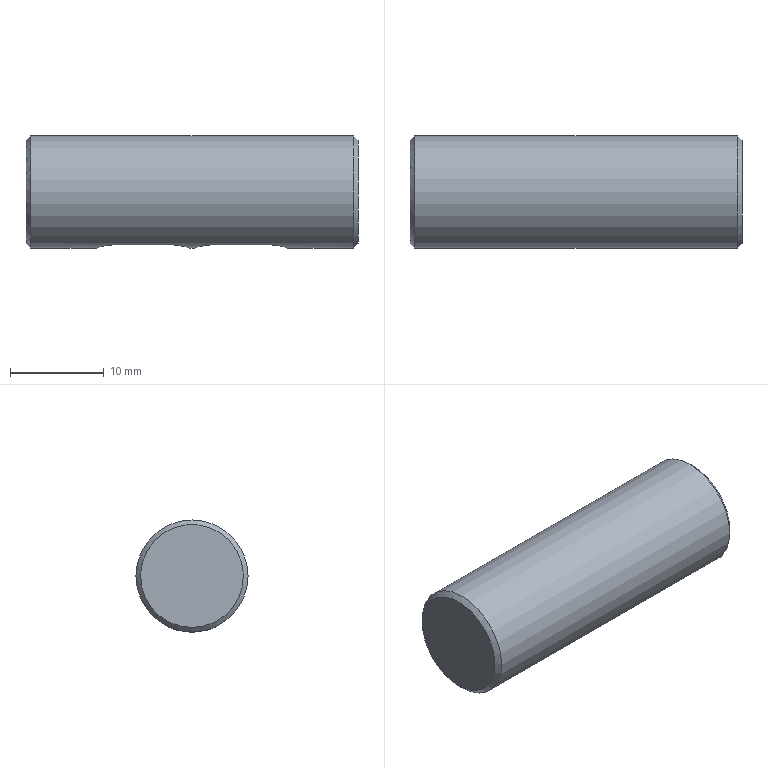Part | NX | features BREP 1 | 1 solid | 15 faces | box 35.5 x 12 x 12 mm | volume 3831 mm3 | plane 8 | cylinder 5 | cone 2 | commonest cylinder face diameters 4 x4 12 x1
STEP:
#1=CARTESIAN_POINT('',(0.5,0.,-6.));
#2=VERTEX_POINT('',#1);
#3=CARTESIAN_POINT('',(0.5,0.,0.));
#4=DIRECTION('',(1.,0.,0.));
#5=DIRECTION('',(0.,0.,-1.));
#6=AXIS2_PLACEMENT_3D('',#3,#4,#5);
#7=CIRCLE('',#6,6.);
#8=EDGE_CURVE('',#2,#2,#7,.T.);
#9=ORIENTED_EDGE('',*,*,#8,.F.);
#10=EDGE_LOOP('',(#9));
#11=FACE_BOUND('',#10,.T.);
#12=CARTESIAN_POINT('',(0.,0.,-5.5));
#13=VERTEX_POINT('',#12);
#14=CARTESIAN_POINT('',(0.,0.,0.));
#15=DIRECTION('',(-1.,0.,0.));
#16=DIRECTION('',(0.,0.,-1.));
#17=AXIS2_PLACEMENT_3D('',#14,#15,#16);
#18=CIRCLE('',#17,5.5);
#19=EDGE_CURVE('',#13,#13,#18,.T.);
#20=ORIENTED_EDGE('',*,*,#19,.F.);
#21=EDGE_LOOP('',(#20));
#22=FACE_BOUND('',#21,.T.);
#23=CARTESIAN_POINT('',(0.,0.,0.));
#24=DIRECTION('',(1.,0.,0.));
#25=DIRECTION('',(0.,0.,-1.));
#26=AXIS2_PLACEMENT_3D('',#23,#24,#25);
#27=CONICAL_SURFACE('',#26,5.5,0.7854);
#28=ADVANCED_FACE('',(#11,#22),#27,.T.);
#29=CARTESIAN_POINT('',(35.,0.,6.));
#30=VERTEX_POINT('',#29);
#31=CARTESIAN_POINT('',(35.,0.,0.));
#32=DIRECTION('',(-1.,0.,0.));
#33=DIRECTION('',(0.,0.,1.));
#34=AXIS2_PLACEMENT_3D('',#31,#32,#33);
#35=CIRCLE('',#34,6.);
#36=EDGE_CURVE('',#30,#30,#35,.T.);
#37=ORIENTED_EDGE('',*,*,#36,.F.);
#38=EDGE_LOOP('',(#37));
#39=FACE_BOUND('',#38,.T.);
#40=CARTESIAN_POINT('',(35.5,0.,5.5));
#41=VERTEX_POINT('',#40);
#42=CARTESIAN_POINT('',(35.5,0.,0.));
#43=DIRECTION('',(1.,0.,0.));
#44=DIRECTION('',(0.,0.,1.));
#45=AXIS2_PLACEMENT_3D('',#42,#43,#44);
#46=CIRCLE('',#45,5.5);
#47=EDGE_CURVE('',#41,#41,#46,.T.);
#48=ORIENTED_EDGE('',*,*,#47,.F.);
#49=EDGE_LOOP('',(#48));
#50=FACE_BOUND('',#49,.T.);
#51=CARTESIAN_POINT('',(35.,0.,0.));
#52=DIRECTION('',(-1.,0.,0.));
#53=DIRECTION('',(0.,0.,1.));
#54=AXIS2_PLACEMENT_3D('',#51,#52,#53);
#55=CONICAL_SURFACE('',#54,6.,0.7854);
#56=ADVANCED_FACE('',(#39,#50),#55,.T.);
#57=CARTESIAN_POINT('',(20.,-2.,-3.5));
#58=VERTEX_POINT('',#57);
#59=CARTESIAN_POINT('',(20.,2.,-3.5));
#60=VERTEX_POINT('',#59);
#61=CARTESIAN_POINT('',(20.,0.,-3.5));
#62=DIRECTION('',(0.,0.,-1.));
#63=DIRECTION('',(1.,0.,0.));
#64=AXIS2_PLACEMENT_3D('',#61,#62,#63);
#65=CIRCLE('',#64,2.);
#66=EDGE_CURVE('',#58,#60,#65,.T.);
#67=ORIENTED_EDGE('',*,*,#66,.F.);
#68=CARTESIAN_POINT('',(20.,-2.,-5.657));
#69=VERTEX_POINT('',#68);
#70=CARTESIAN_POINT('',(20.,-2.,-3.5));
#71=DIRECTION('',(0.,0.,-1.));
#72=VECTOR('',#71,1000.);
#73=LINE('',#70,#72);
#74=EDGE_CURVE('',#58,#69,#73,.T.);
#75=ORIENTED_EDGE('',*,*,#74,.T.);
#76=CARTESIAN_POINT('',(20.,2.,-5.657));
#77=VERTEX_POINT('',#76);
#78=CARTESIAN_POINT('',(20.,2.,-5.657));
#79=CARTESIAN_POINT('',(19.467,2.,-5.657));
#80=CARTESIAN_POINT('',(18.438,1.567,-5.833));
#81=CARTESIAN_POINT('',(17.781,0.003461,-6.083));
#82=CARTESIAN_POINT('',(18.437,-1.568,-5.834));
#83=CARTESIAN_POINT('',(19.467,-2.,-5.657));
#84=CARTESIAN_POINT('',(20.,-2.,-5.657));
#85=B_SPLINE_CURVE_WITH_KNOTS('',3,(#78,#79,#80,#81,#82,#83,#84),.UNSPECIFIED.,.F.,.F.,(4,1,1,1,4),(0.,0.001574,0.003148,0.004722,0.006296),.UNSPECIFIED.);
#86=EDGE_CURVE('',#77,#69,#85,.T.);
#87=ORIENTED_EDGE('',*,*,#86,.F.);
#88=CARTESIAN_POINT('',(20.,2.,-3.5));
#89=DIRECTION('',(0.,0.,-1.));
#90=VECTOR('',#89,1000.);
#91=LINE('',#88,#90);
#92=EDGE_CURVE('',#60,#77,#91,.T.);
#93=ORIENTED_EDGE('',*,*,#92,.F.);
#94=EDGE_LOOP('',(#67,#75,#87,#93));
#95=FACE_BOUND('',#94,.T.);
#96=CARTESIAN_POINT('',(20.,0.,-3.5));
#97=DIRECTION('',(0.,0.,-1.));
#98=DIRECTION('',(-1.,0.,0.));
#99=AXIS2_PLACEMENT_3D('',#96,#97,#98);
#100=CYLINDRICAL_SURFACE('',#99,2.);
#101=ADVANCED_FACE('',(#95),#100,.F.);
#102=CARTESIAN_POINT('',(9.5,-2.,-3.5));
#103=VERTEX_POINT('',#102);
#104=CARTESIAN_POINT('',(9.5,2.,-3.5));
#105=VERTEX_POINT('',#104);
#106=CARTESIAN_POINT('',(9.5,0.,-3.5));
#107=DIRECTION('',(0.,0.,-1.));
#108=DIRECTION('',(1.,0.,0.));
#109=AXIS2_PLACEMENT_3D('',#106,#107,#108);
#110=CIRCLE('',#109,2.);
#111=EDGE_CURVE('',#103,#105,#110,.T.);
#112=ORIENTED_EDGE('',*,*,#111,.F.);
#113=CARTESIAN_POINT('',(9.5,-2.,-5.657));
#114=VERTEX_POINT('',#113);
#115=CARTESIAN_POINT('',(9.5,-2.,-3.5));
#116=DIRECTION('',(0.,0.,-1.));
#117=VECTOR('',#116,1000.);
#118=LINE('',#115,#117);
#119=EDGE_CURVE('',#103,#114,#118,.T.);
#120=ORIENTED_EDGE('',*,*,#119,.T.);
#121=CARTESIAN_POINT('',(9.5,2.,-5.657));
#122=VERTEX_POINT('',#121);
#123=CARTESIAN_POINT('',(9.5,2.,-5.657));
#124=CARTESIAN_POINT('',(8.967,2.,-5.657));
#125=CARTESIAN_POINT('',(7.938,1.567,-5.833));
#126=CARTESIAN_POINT('',(7.281,0.003461,-6.083));
#127=CARTESIAN_POINT('',(7.937,-1.568,-5.834));
#128=CARTESIAN_POINT('',(8.967,-2.,-5.657));
#129=CARTESIAN_POINT('',(9.5,-2.,-5.657));
#130=B_SPLINE_CURVE_WITH_KNOTS('',3,(#123,#124,#125,#126,#127,#128,#129),.UNSPECIFIED.,.F.,.F.,(4,1,1,1,4),(0.,0.001574,0.003148,0.004722,0.006296),.UNSPECIFIED.);
#131=EDGE_CURVE('',#122,#114,#130,.T.);
#132=ORIENTED_EDGE('',*,*,#131,.F.);
#133=CARTESIAN_POINT('',(9.5,2.,-3.5));
#134=DIRECTION('',(0.,0.,-1.));
#135=VECTOR('',#134,1000.);
#136=LINE('',#133,#135);
#137=EDGE_CURVE('',#105,#122,#136,.T.);
#138=ORIENTED_EDGE('',*,*,#137,.F.);
#139=EDGE_LOOP('',(#112,#120,#132,#138));
#140=FACE_BOUND('',#139,.T.);
#141=CARTESIAN_POINT('',(9.5,0.,-3.5));
#142=DIRECTION('',(0.,0.,-1.));
#143=DIRECTION('',(-1.,0.,0.));
#144=AXIS2_PLACEMENT_3D('',#141,#142,#143);
#145=CYLINDRICAL_SURFACE('',#144,2.);
#146=ADVANCED_FACE('',(#140),#145,.F.);
#147=ORIENTED_EDGE('',*,*,#8,.T.);
#148=EDGE_LOOP('',(#147));
#149=FACE_BOUND('',#148,.T.);
#150=ORIENTED_EDGE('',*,*,#36,.T.);
#151=EDGE_LOOP('',(#150));
#152=FACE_BOUND('',#151,.T.);
#153=CARTESIAN_POINT('',(15.5,-2.,-5.657));
#154=VERTEX_POINT('',#153);
#155=CARTESIAN_POINT('',(0.,-2.,-5.657));
#156=DIRECTION('',(1.,0.,0.));
#157=VECTOR('',#156,1000.);
#158=LINE('',#155,#157);
#159=EDGE_CURVE('',#114,#154,#158,.T.);
#160=ORIENTED_EDGE('',*,*,#159,.T.);
#161=CARTESIAN_POINT('',(15.5,2.,-5.657));
#162=VERTEX_POINT('',#161);
#163=CARTESIAN_POINT('',(15.5,-2.,-5.657));
#164=CARTESIAN_POINT('',(16.033,-2.,-5.657));
#165=CARTESIAN_POINT('',(17.062,-1.567,-5.833));
#166=CARTESIAN_POINT('',(17.719,-0.003461,-6.083));
#167=CARTESIAN_POINT('',(17.063,1.568,-5.834));
#168=CARTESIAN_POINT('',(16.033,2.,-5.657));
#169=CARTESIAN_POINT('',(15.5,2.,-5.657));
#170=B_SPLINE_CURVE_WITH_KNOTS('',3,(#163,#164,#165,#166,#167,#168,#169),.UNSPECIFIED.,.F.,.F.,(4,1,1,1,4),(0.,0.001574,0.003148,0.004722,0.006296),.UNSPECIFIED.);
#171=EDGE_CURVE('',#154,#162,#170,.T.);
#172=ORIENTED_EDGE('',*,*,#171,.T.);
#173=CARTESIAN_POINT('',(0.,2.,-5.657));
#174=DIRECTION('',(-1.,0.,0.));
#175=VECTOR('',#174,1000.);
#176=LINE('',#173,#175);
#177=EDGE_CURVE('',#162,#122,#176,.T.);
#178=ORIENTED_EDGE('',*,*,#177,.T.);
#179=ORIENTED_EDGE('',*,*,#131,.T.);
#180=EDGE_LOOP('',(#160,#172,#178,#179));
#181=FACE_BOUND('',#180,.T.);
#182=ORIENTED_EDGE('',*,*,#86,.T.);
#183=CARTESIAN_POINT('',(26.,-2.,-5.657));
#184=VERTEX_POINT('',#183);
#185=CARTESIAN_POINT('',(0.,-2.,-5.657));
#186=DIRECTION('',(1.,0.,0.));
#187=VECTOR('',#186,1000.);
#188=LINE('',#185,#187);
#189=EDGE_CURVE('',#69,#184,#188,.T.);
#190=ORIENTED_EDGE('',*,*,#189,.T.);
#191=CARTESIAN_POINT('',(26.,2.,-5.657));
#192=VERTEX_POINT('',#191);
#193=CARTESIAN_POINT('',(26.,-2.,-5.657));
#194=CARTESIAN_POINT('',(26.533,-2.,-5.657));
#195=CARTESIAN_POINT('',(27.562,-1.567,-5.833));
#196=CARTESIAN_POINT('',(28.219,-0.003461,-6.083));
#197=CARTESIAN_POINT('',(27.563,1.568,-5.834));
#198=CARTESIAN_POINT('',(26.533,2.,-5.657));
#199=CARTESIAN_POINT('',(26.,2.,-5.657));
#200=B_SPLINE_CURVE_WITH_KNOTS('',3,(#193,#194,#195,#196,#197,#198,#199),.UNSPECIFIED.,.F.,.F.,(4,1,1,1,4),(0.,0.001574,0.003148,0.004722,0.006296),.UNSPECIFIED.);
#201=EDGE_CURVE('',#184,#192,#200,.T.);
#202=ORIENTED_EDGE('',*,*,#201,.T.);
#203=CARTESIAN_POINT('',(0.,2.,-5.657));
#204=DIRECTION('',(-1.,0.,0.));
#205=VECTOR('',#204,1000.);
#206=LINE('',#203,#205);
#207=EDGE_CURVE('',#192,#77,#206,.T.);
#208=ORIENTED_EDGE('',*,*,#207,.T.);
#209=EDGE_LOOP('',(#182,#190,#202,#208));
#210=FACE_BOUND('',#209,.T.);
#211=CARTESIAN_POINT('',(0.,0.,0.));
#212=DIRECTION('',(-1.,0.,0.));
#213=DIRECTION('',(0.,0.,1.));
#214=AXIS2_PLACEMENT_3D('',#211,#212,#213);
#215=CYLINDRICAL_SURFACE('',#214,6.);
#216=ADVANCED_FACE('',(#149,#152,#181,#210),#215,.T.);
#217=ORIENTED_EDGE('',*,*,#47,.T.);
#218=EDGE_LOOP('',(#217));
#219=FACE_BOUND('',#218,.T.);
#220=CARTESIAN_POINT('',(35.5,0.,0.));
#221=DIRECTION('',(-1.,0.,0.));
#222=DIRECTION('',(0.,0.,1.));
#223=AXIS2_PLACEMENT_3D('',#220,#221,#222);
#224=PLANE('',#223);
#225=ADVANCED_FACE('',(#219),#224,.F.);
#226=ORIENTED_EDGE('',*,*,#19,.T.);
#227=EDGE_LOOP('',(#226));
#228=FACE_BOUND('',#227,.T.);
#229=CARTESIAN_POINT('',(0.,6.,0.));
#230=DIRECTION('',(1.,0.,0.));
#231=DIRECTION('',(0.,0.,-1.));
#232=AXIS2_PLACEMENT_3D('',#229,#230,#231);
#233=PLANE('',#232);
#234=ADVANCED_FACE('',(#228),#233,.F.);
#235=CARTESIAN_POINT('',(15.5,-2.,-3.5));
#236=VERTEX_POINT('',#235);
#237=CARTESIAN_POINT('',(15.5,-2.,-3.5));
#238=DIRECTION('',(0.,0.,-1.));
#239=VECTOR('',#238,1000.);
#240=LINE('',#237,#239);
#241=EDGE_CURVE('',#236,#154,#240,.T.);
#242=ORIENTED_EDGE('',*,*,#241,.F.);
#243=CARTESIAN_POINT('',(15.5,2.,-3.5));
#244=VERTEX_POINT('',#243);
#245=CARTESIAN_POINT('',(15.5,0.,-3.5));
#246=DIRECTION('',(0.,0.,-1.));
#247=DIRECTION('',(-1.,0.,0.));
#248=AXIS2_PLACEMENT_3D('',#245,#246,#247);
#249=CIRCLE('',#248,2.);
#250=EDGE_CURVE('',#244,#236,#249,.T.);
#251=ORIENTED_EDGE('',*,*,#250,.F.);
#252=CARTESIAN_POINT('',(15.5,2.,-3.5));
#253=DIRECTION('',(0.,0.,-1.));
#254=VECTOR('',#253,1000.);
#255=LINE('',#252,#254);
#256=EDGE_CURVE('',#244,#162,#255,.T.);
#257=ORIENTED_EDGE('',*,*,#256,.T.);
#258=ORIENTED_EDGE('',*,*,#171,.F.);
#259=EDGE_LOOP('',(#242,#251,#257,#258));
#260=FACE_BOUND('',#259,.T.);
#261=CARTESIAN_POINT('',(15.5,0.,-3.5));
#262=DIRECTION('',(0.,0.,-1.));
#263=DIRECTION('',(-1.,0.,0.));
#264=AXIS2_PLACEMENT_3D('',#261,#262,#263);
#265=CYLINDRICAL_SURFACE('',#264,2.);
#266=ADVANCED_FACE('',(#260),#265,.F.);
#267=ORIENTED_EDGE('',*,*,#256,.F.);
#268=CARTESIAN_POINT('',(15.5,2.,-3.5));
#269=DIRECTION('',(1.,0.,0.));
#270=VECTOR('',#269,1000.);
#271=LINE('',#268,#270);
#272=EDGE_CURVE('',#105,#244,#271,.T.);
#273=ORIENTED_EDGE('',*,*,#272,.F.);
#274=ORIENTED_EDGE('',*,*,#137,.T.);
#275=ORIENTED_EDGE('',*,*,#177,.F.);
#276=EDGE_LOOP('',(#267,#273,#274,#275));
#277=FACE_BOUND('',#276,.T.);
#278=CARTESIAN_POINT('',(15.5,2.,-3.5));
#279=DIRECTION('',(0.,1.,0.));
#280=DIRECTION('',(-1.,0.,0.));
#281=AXIS2_PLACEMENT_3D('',#278,#279,#280);
#282=PLANE('',#281);
#283=ADVANCED_FACE('',(#277),#282,.F.);
#284=ORIENTED_EDGE('',*,*,#119,.F.);
#285=CARTESIAN_POINT('',(15.5,-2.,-3.5));
#286=DIRECTION('',(-1.,0.,0.));
#287=VECTOR('',#286,1000.);
#288=LINE('',#285,#287);
#289=EDGE_CURVE('',#236,#103,#288,.T.);
#290=ORIENTED_EDGE('',*,*,#289,.F.);
#291=ORIENTED_EDGE('',*,*,#241,.T.);
#292=ORIENTED_EDGE('',*,*,#159,.F.);
#293=EDGE_LOOP('',(#284,#290,#291,#292));
#294=FACE_BOUND('',#293,.T.);
#295=CARTESIAN_POINT('',(15.5,-2.,-3.5));
#296=DIRECTION('',(0.,-1.,0.));
#297=DIRECTION('',(0.,0.,-1.));
#298=AXIS2_PLACEMENT_3D('',#295,#296,#297);
#299=PLANE('',#298);
#300=ADVANCED_FACE('',(#294),#299,.F.);
#301=ORIENTED_EDGE('',*,*,#250,.T.);
#302=ORIENTED_EDGE('',*,*,#289,.T.);
#303=ORIENTED_EDGE('',*,*,#111,.T.);
#304=ORIENTED_EDGE('',*,*,#272,.T.);
#305=EDGE_LOOP('',(#301,#302,#303,#304));
#306=FACE_BOUND('',#305,.T.);
#307=CARTESIAN_POINT('',(15.5,0.,-3.5));
#308=DIRECTION('',(0.,0.,-1.));
#309=DIRECTION('',(-1.,0.,0.));
#310=AXIS2_PLACEMENT_3D('',#307,#308,#309);
#311=PLANE('',#310);
#312=ADVANCED_FACE('',(#306),#311,.T.);
#313=CARTESIAN_POINT('',(26.,-2.,-3.5));
#314=VERTEX_POINT('',#313);
#315=CARTESIAN_POINT('',(26.,-2.,-3.5));
#316=DIRECTION('',(0.,0.,-1.));
#317=VECTOR('',#316,1000.);
#318=LINE('',#315,#317);
#319=EDGE_CURVE('',#314,#184,#318,.T.);
#320=ORIENTED_EDGE('',*,*,#319,.F.);
#321=CARTESIAN_POINT('',(26.,2.,-3.5));
#322=VERTEX_POINT('',#321);
#323=CARTESIAN_POINT('',(26.,0.,-3.5));
#324=DIRECTION('',(0.,0.,-1.));
#325=DIRECTION('',(-1.,0.,0.));
#326=AXIS2_PLACEMENT_3D('',#323,#324,#325);
#327=CIRCLE('',#326,2.);
#328=EDGE_CURVE('',#322,#314,#327,.T.);
#329=ORIENTED_EDGE('',*,*,#328,.F.);
#330=CARTESIAN_POINT('',(26.,2.,-3.5));
#331=DIRECTION('',(0.,0.,-1.));
#332=VECTOR('',#331,1000.);
#333=LINE('',#330,#332);
#334=EDGE_CURVE('',#322,#192,#333,.T.);
#335=ORIENTED_EDGE('',*,*,#334,.T.);
#336=ORIENTED_EDGE('',*,*,#201,.F.);
#337=EDGE_LOOP('',(#320,#329,#335,#336));
#338=FACE_BOUND('',#337,.T.);
#339=CARTESIAN_POINT('',(26.,0.,-3.5));
#340=DIRECTION('',(0.,0.,-1.));
#341=DIRECTION('',(-1.,0.,0.));
#342=AXIS2_PLACEMENT_3D('',#339,#340,#341);
#343=CYLINDRICAL_SURFACE('',#342,2.);
#344=ADVANCED_FACE('',(#338),#343,.F.);
#345=ORIENTED_EDGE('',*,*,#334,.F.);
#346=CARTESIAN_POINT('',(26.,2.,-3.5));
#347=DIRECTION('',(1.,0.,0.));
#348=VECTOR('',#347,1000.);
#349=LINE('',#346,#348);
#350=EDGE_CURVE('',#60,#322,#349,.T.);
#351=ORIENTED_EDGE('',*,*,#350,.F.);
#352=ORIENTED_EDGE('',*,*,#92,.T.);
#353=ORIENTED_EDGE('',*,*,#207,.F.);
#354=EDGE_LOOP('',(#345,#351,#352,#353));
#355=FACE_BOUND('',#354,.T.);
#356=CARTESIAN_POINT('',(26.,2.,-3.5));
#357=DIRECTION('',(0.,1.,0.));
#358=DIRECTION('',(0.,0.,1.));
#359=AXIS2_PLACEMENT_3D('',#356,#357,#358);
#360=PLANE('',#359);
#361=ADVANCED_FACE('',(#355),#360,.F.);
#362=ORIENTED_EDGE('',*,*,#74,.F.);
#363=CARTESIAN_POINT('',(26.,-2.,-3.5));
#364=DIRECTION('',(-1.,0.,0.));
#365=VECTOR('',#364,1000.);
#366=LINE('',#363,#365);
#367=EDGE_CURVE('',#314,#58,#366,.T.);
#368=ORIENTED_EDGE('',*,*,#367,.F.);
#369=ORIENTED_EDGE('',*,*,#319,.T.);
#370=ORIENTED_EDGE('',*,*,#189,.F.);
#371=EDGE_LOOP('',(#362,#368,#369,#370));
#372=FACE_BOUND('',#371,.T.);
#373=CARTESIAN_POINT('',(26.,-2.,-3.5));
#374=DIRECTION('',(0.,-1.,0.));
#375=DIRECTION('',(0.,0.,-1.));
#376=AXIS2_PLACEMENT_3D('',#373,#374,#375);
#377=PLANE('',#376);
#378=ADVANCED_FACE('',(#372),#377,.F.);
#379=ORIENTED_EDGE('',*,*,#328,.T.);
#380=ORIENTED_EDGE('',*,*,#367,.T.);
#381=ORIENTED_EDGE('',*,*,#66,.T.);
#382=ORIENTED_EDGE('',*,*,#350,.T.);
#383=EDGE_LOOP('',(#379,#380,#381,#382));
#384=FACE_BOUND('',#383,.T.);
#385=CARTESIAN_POINT('',(26.,0.,-3.5));
#386=DIRECTION('',(0.,0.,-1.));
#387=DIRECTION('',(-1.,0.,0.));
#388=AXIS2_PLACEMENT_3D('',#385,#386,#387);
#389=PLANE('',#388);
#390=ADVANCED_FACE('',(#384),#389,.T.);
#391=CLOSED_SHELL('',(#28,#56,#101,#146,#216,#225,#234,#266,#283,#300,#312,#344,#361,#378,#390));
#392=MANIFOLD_SOLID_BREP('',#391);
#393=(LENGTH_UNIT()NAMED_UNIT(*)SI_UNIT(.MILLI.,.METRE.));
#394=UNCERTAINTY_MEASURE_WITH_UNIT(LENGTH_MEASURE(0.0508),#393,'','');
#395=(NAMED_UNIT(*)PLANE_ANGLE_UNIT()SI_UNIT($,.RADIAN.));
#396=(NAMED_UNIT(*)SI_UNIT($,.STERADIAN.)SOLID_ANGLE_UNIT());
#397=(GEOMETRIC_REPRESENTATION_CONTEXT(3)GLOBAL_UNCERTAINTY_ASSIGNED_CONTEXT((#394))GLOBAL_UNIT_ASSIGNED_CONTEXT((#393,#395,#396))REPRESENTATION_CONTEXT('',''));
#398=ADVANCED_BREP_SHAPE_REPRESENTATION('',(#392),#397);